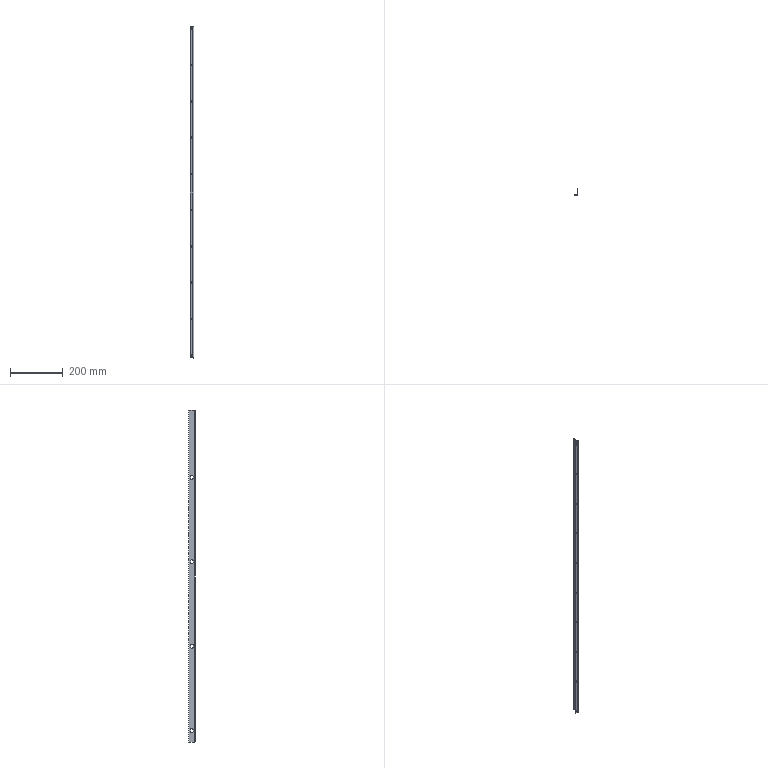Part | NX | features solid 2 | 1 solid | 54 faces | box 15 x 25 x 1259 mm | volume 90750 mm3 | cylinder 34 | plane 20 | commonest cylinder face diameters 6 x20 9 x12 4 x1 8 x1